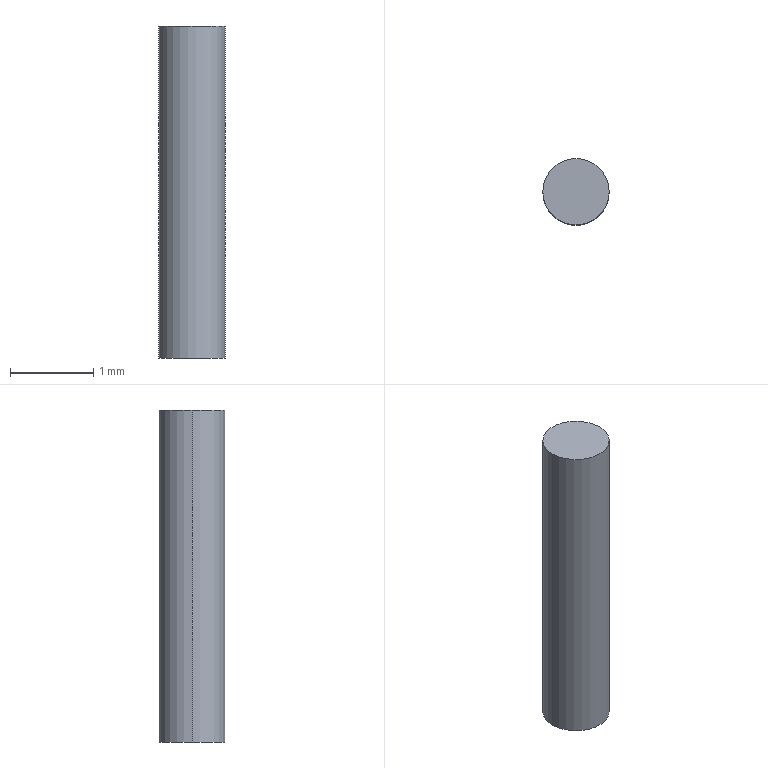Part | STEP file | RJ-USIO-V1_2-220411_13 | 1 solid | 4 faces | box 0.8 x 0.8 x 4 mm | volume 2.011 mm3 | cylinder 2 | plane 2 | commonest cylinder face diameters 0.8 x2
STEP:
#1=CARTESIAN_POINT('',(0.,0.,0.));
#2=DIRECTION('',(0.,0.,1.));
#3=DIRECTION('',(1.,0.,0.));
#4=AXIS2_PLACEMENT_3D('',#1,#2,#3);
#5=CARTESIAN_POINT('',(42.7,30.62,0.000002004));
#6=VERTEX_POINT('',#5);
#7=CARTESIAN_POINT('',(42.7,30.62,-4.));
#8=VERTEX_POINT('',#7);
#9=CARTESIAN_POINT('',(42.7,30.62,0.000002004));
#10=DIRECTION('',(0.,0.,-1.));
#11=VECTOR('',#10,1.);
#12=LINE('',#9,#11);
#13=CARTESIAN_POINT('',(42.3,30.62,-4.));
#14=DIRECTION('',(0.,0.,-1.));
#15=DIRECTION('',(1.,0.000000087,0.));
#16=AXIS2_PLACEMENT_3D('',#13,#14,#15);
#17=CYLINDRICAL_SURFACE('',#16,0.4);
#18=CARTESIAN_POINT('',(6.283,-4.));
#19=DIRECTION('',(0.,1.));
#20=VECTOR('',#19,1.);
#21=LINE('',#18,#20);
#22=(GEOMETRIC_REPRESENTATION_CONTEXT(2)PARAMETRIC_REPRESENTATION_CONTEXT()REPRESENTATION_CONTEXT('',''));
#23=DEFINITIONAL_REPRESENTATION('',(#21),#22);
#24=PCURVE('',#17,#23);
#25=CARTESIAN_POINT('',(42.3,30.62,-4.));
#26=DIRECTION('',(0.,0.,-1.));
#27=DIRECTION('',(1.,0.000000087,0.));
#28=AXIS2_PLACEMENT_3D('',#25,#26,#27);
#29=CYLINDRICAL_SURFACE('',#28,0.4);
#30=CARTESIAN_POINT('',(0.,-4.));
#31=DIRECTION('',(0.,1.));
#32=VECTOR('',#31,1.);
#33=LINE('',#30,#32);
#34=(GEOMETRIC_REPRESENTATION_CONTEXT(2)PARAMETRIC_REPRESENTATION_CONTEXT()REPRESENTATION_CONTEXT('',''));
#35=DEFINITIONAL_REPRESENTATION('',(#33),#34);
#36=PCURVE('',#29,#35);
#37=SURFACE_CURVE('',#12,(#24,#36),.PCURVE_S1.);
#38=EDGE_CURVE('',#6,#8,#37,.T.);
#39=ORIENTED_EDGE('',*,*,#38,.T.);
#40=CARTESIAN_POINT('',(41.9,30.62,-4.));
#41=VERTEX_POINT('',#40);
#42=CARTESIAN_POINT('',(42.3,30.62,-4.));
#43=DIRECTION('',(0.,0.,-1.));
#44=DIRECTION('',(-1.,-0.000000087,0.));
#45=AXIS2_PLACEMENT_3D('',#42,#43,#44);
#46=CIRCLE('',#45,0.4);
#47=CARTESIAN_POINT('',(3.142,0.));
#48=DIRECTION('',(1.,0.));
#49=VECTOR('',#48,1.);
#50=LINE('',#47,#49);
#51=(GEOMETRIC_REPRESENTATION_CONTEXT(2)PARAMETRIC_REPRESENTATION_CONTEXT()REPRESENTATION_CONTEXT('',''));
#52=DEFINITIONAL_REPRESENTATION('',(#50),#51);
#53=PCURVE('',#17,#52);
#54=CARTESIAN_POINT('',(41.9,30.62,-4.));
#55=DIRECTION('',(0.,0.,-1.));
#56=DIRECTION('',(-1.,-0.000000087,0.));
#57=AXIS2_PLACEMENT_3D('',#54,#55,#56);
#58=PLANE('',#57);
#59=CARTESIAN_POINT('',(-0.4,0.));
#60=DIRECTION('',(1.,0.));
#61=AXIS2_PLACEMENT_2D('',#59,#60);
#62=CIRCLE('',#61,0.4);
#63=(GEOMETRIC_REPRESENTATION_CONTEXT(2)PARAMETRIC_REPRESENTATION_CONTEXT()REPRESENTATION_CONTEXT('',''));
#64=DEFINITIONAL_REPRESENTATION('',(#62),#63);
#65=PCURVE('',#58,#64);
#66=SURFACE_CURVE('',#46,(#53,#65),.PCURVE_S1.);
#67=EDGE_CURVE('',#41,#8,#66,.T.);
#68=ORIENTED_EDGE('',*,*,#67,.F.);
#69=CARTESIAN_POINT('',(41.9,30.62,0.000002004));
#70=VERTEX_POINT('',#69);
#71=CARTESIAN_POINT('',(41.9,30.62,0.000002004));
#72=DIRECTION('',(0.,0.,-1.));
#73=VECTOR('',#72,1.);
#74=LINE('',#71,#73);
#75=CARTESIAN_POINT('',(3.142,-4.));
#76=DIRECTION('',(0.,1.));
#77=VECTOR('',#76,1.);
#78=LINE('',#75,#77);
#79=(GEOMETRIC_REPRESENTATION_CONTEXT(2)PARAMETRIC_REPRESENTATION_CONTEXT()REPRESENTATION_CONTEXT('',''));
#80=DEFINITIONAL_REPRESENTATION('',(#78),#79);
#81=PCURVE('',#17,#80);
#82=CARTESIAN_POINT('',(3.142,-4.));
#83=DIRECTION('',(0.,1.));
#84=VECTOR('',#83,1.);
#85=LINE('',#82,#84);
#86=(GEOMETRIC_REPRESENTATION_CONTEXT(2)PARAMETRIC_REPRESENTATION_CONTEXT()REPRESENTATION_CONTEXT('',''));
#87=DEFINITIONAL_REPRESENTATION('',(#85),#86);
#88=PCURVE('',#29,#87);
#89=SURFACE_CURVE('',#74,(#81,#88),.PCURVE_S1.);
#90=EDGE_CURVE('',#70,#41,#89,.T.);
#91=ORIENTED_EDGE('',*,*,#90,.F.);
#92=CARTESIAN_POINT('',(42.3,30.62,0.000002004));
#93=DIRECTION('',(0.,0.,1.));
#94=DIRECTION('',(1.,0.000000087,0.));
#95=AXIS2_PLACEMENT_3D('',#92,#93,#94);
#96=CIRCLE('',#95,0.4);
#97=CARTESIAN_POINT('',(6.283,-4.));
#98=DIRECTION('',(-1.,0.));
#99=VECTOR('',#98,1.);
#100=LINE('',#97,#99);
#101=(GEOMETRIC_REPRESENTATION_CONTEXT(2)PARAMETRIC_REPRESENTATION_CONTEXT()REPRESENTATION_CONTEXT('',''));
#102=DEFINITIONAL_REPRESENTATION('',(#100),#101);
#103=PCURVE('',#17,#102);
#104=CARTESIAN_POINT('',(41.9,30.62,0.000002004));
#105=DIRECTION('',(0.,0.,-1.));
#106=DIRECTION('',(-1.,-0.000000087,0.));
#107=AXIS2_PLACEMENT_3D('',#104,#105,#106);
#108=PLANE('',#107);
#109=CARTESIAN_POINT('',(-0.8,0.));
#110=CARTESIAN_POINT('',(-0.8,0.6928));
#111=CARTESIAN_POINT('',(-0.2,0.3464));
#112=CARTESIAN_POINT('',(0.4,0.));
#113=CARTESIAN_POINT('',(-0.2,-0.3464));
#114=CARTESIAN_POINT('',(-0.8,-0.6928));
#115=CARTESIAN_POINT('',(-0.8,0.));
#116=(BOUNDED_CURVE()B_SPLINE_CURVE(2,(#109,#110,#111,#112,#113,#114,#115),.UNSPECIFIED.,.T.,.F.)B_SPLINE_CURVE_WITH_KNOTS((1,2,2,2,2,1),(-2.094,0.,2.094,4.189,6.283,8.378),.UNSPECIFIED.)CURVE()GEOMETRIC_REPRESENTATION_ITEM()RATIONAL_B_SPLINE_CURVE((1.,0.5,1.,0.5,1.,0.5,1.))REPRESENTATION_ITEM(''));
#117=(GEOMETRIC_REPRESENTATION_CONTEXT(2)PARAMETRIC_REPRESENTATION_CONTEXT()REPRESENTATION_CONTEXT('',''));
#118=DEFINITIONAL_REPRESENTATION('',(#116),#117);
#119=PCURVE('',#108,#118);
#120=SURFACE_CURVE('',#96,(#103,#119),.PCURVE_S1.);
#121=EDGE_CURVE('',#6,#70,#120,.T.);
#122=ORIENTED_EDGE('',*,*,#121,.F.);
#123=EDGE_LOOP('',(#39,#68,#91,#122));
#124=FACE_BOUND('',#123,.T.);
#125=ADVANCED_FACE('',(#124),#17,.T.);
#126=CARTESIAN_POINT('',(42.3,30.62,0.000002004));
#127=DIRECTION('',(0.,0.,1.));
#128=DIRECTION('',(-1.,-0.000000087,0.));
#129=AXIS2_PLACEMENT_3D('',#126,#127,#128);
#130=CIRCLE('',#129,0.4);
#131=CARTESIAN_POINT('',(0.,0.));
#132=CARTESIAN_POINT('',(0.,-0.6928));
#133=CARTESIAN_POINT('',(-0.6,-0.3464));
#134=CARTESIAN_POINT('',(-1.2,0.));
#135=CARTESIAN_POINT('',(-0.6,0.3464));
#136=CARTESIAN_POINT('',(0.,0.6928));
#137=CARTESIAN_POINT('',(0.,0.));
#138=(BOUNDED_CURVE()B_SPLINE_CURVE(2,(#131,#132,#133,#134,#135,#136,#137),.UNSPECIFIED.,.T.,.F.)B_SPLINE_CURVE_WITH_KNOTS((1,2,2,2,2,1),(-2.094,0.,2.094,4.189,6.283,8.378),.UNSPECIFIED.)CURVE()GEOMETRIC_REPRESENTATION_ITEM()RATIONAL_B_SPLINE_CURVE((1.,0.5,1.,0.5,1.,0.5,1.))REPRESENTATION_ITEM(''));
#139=(GEOMETRIC_REPRESENTATION_CONTEXT(2)PARAMETRIC_REPRESENTATION_CONTEXT()REPRESENTATION_CONTEXT('',''));
#140=DEFINITIONAL_REPRESENTATION('',(#138),#139);
#141=PCURVE('',#108,#140);
#142=CARTESIAN_POINT('',(3.142,-4.));
#143=DIRECTION('',(-1.,0.));
#144=VECTOR('',#143,1.);
#145=LINE('',#142,#144);
#146=(GEOMETRIC_REPRESENTATION_CONTEXT(2)PARAMETRIC_REPRESENTATION_CONTEXT()REPRESENTATION_CONTEXT('',''));
#147=DEFINITIONAL_REPRESENTATION('',(#145),#146);
#148=PCURVE('',#29,#147);
#149=SURFACE_CURVE('',#130,(#141,#148),.PCURVE_S1.);
#150=EDGE_CURVE('',#70,#6,#149,.T.);
#151=ORIENTED_EDGE('',*,*,#150,.F.);
#152=ORIENTED_EDGE('',*,*,#121,.F.);
#153=EDGE_LOOP('',(#151,#152));
#154=FACE_BOUND('',#153,.F.);
#155=ADVANCED_FACE('',(#154),#108,.F.);
#156=ORIENTED_EDGE('',*,*,#150,.F.);
#157=ORIENTED_EDGE('',*,*,#90,.T.);
#158=CARTESIAN_POINT('',(42.3,30.62,-4.));
#159=DIRECTION('',(0.,0.,-1.));
#160=DIRECTION('',(1.,0.000000087,0.));
#161=AXIS2_PLACEMENT_3D('',#158,#159,#160);
#162=CIRCLE('',#161,0.4);
#163=CARTESIAN_POINT('',(0.,0.));
#164=DIRECTION('',(1.,0.));
#165=VECTOR('',#164,1.);
#166=LINE('',#163,#165);
#167=(GEOMETRIC_REPRESENTATION_CONTEXT(2)PARAMETRIC_REPRESENTATION_CONTEXT()REPRESENTATION_CONTEXT('',''));
#168=DEFINITIONAL_REPRESENTATION('',(#166),#167);
#169=PCURVE('',#29,#168);
#170=CARTESIAN_POINT('',(-0.4,0.));
#171=DIRECTION('',(-1.,0.));
#172=AXIS2_PLACEMENT_2D('',#170,#171);
#173=CIRCLE('',#172,0.4);
#174=(GEOMETRIC_REPRESENTATION_CONTEXT(2)PARAMETRIC_REPRESENTATION_CONTEXT()REPRESENTATION_CONTEXT('',''));
#175=DEFINITIONAL_REPRESENTATION('',(#173),#174);
#176=PCURVE('',#58,#175);
#177=SURFACE_CURVE('',#162,(#169,#176),.PCURVE_S1.);
#178=EDGE_CURVE('',#8,#41,#177,.T.);
#179=ORIENTED_EDGE('',*,*,#178,.F.);
#180=ORIENTED_EDGE('',*,*,#38,.F.);
#181=EDGE_LOOP('',(#156,#157,#179,#180));
#182=FACE_BOUND('',#181,.T.);
#183=ADVANCED_FACE('',(#182),#29,.T.);
#184=ORIENTED_EDGE('',*,*,#178,.F.);
#185=ORIENTED_EDGE('',*,*,#67,.F.);
#186=EDGE_LOOP('',(#184,#185));
#187=FACE_BOUND('',#186,.F.);
#188=ADVANCED_FACE('',(#187),#58,.T.);
#189=CLOSED_SHELL('',(#125,#155,#183,#188));
#190=MANIFOLD_SOLID_BREP('',#189);
#191=(LENGTH_UNIT()NAMED_UNIT(*)SI_UNIT(.MILLI.,.METRE.));
#192=UNCERTAINTY_MEASURE_WITH_UNIT(LENGTH_MEASURE(0.0000001),#191,'','');
#193=(NAMED_UNIT(*)PLANE_ANGLE_UNIT()SI_UNIT($,.RADIAN.));
#194=(NAMED_UNIT(*)SI_UNIT($,.STERADIAN.)SOLID_ANGLE_UNIT());
#195=(GEOMETRIC_REPRESENTATION_CONTEXT(3)GLOBAL_UNCERTAINTY_ASSIGNED_CONTEXT((#192))GLOBAL_UNIT_ASSIGNED_CONTEXT((#191,#193,#194))REPRESENTATION_CONTEXT('',''));
#196=ADVANCED_BREP_SHAPE_REPRESENTATION('',(#4,#190),#195);